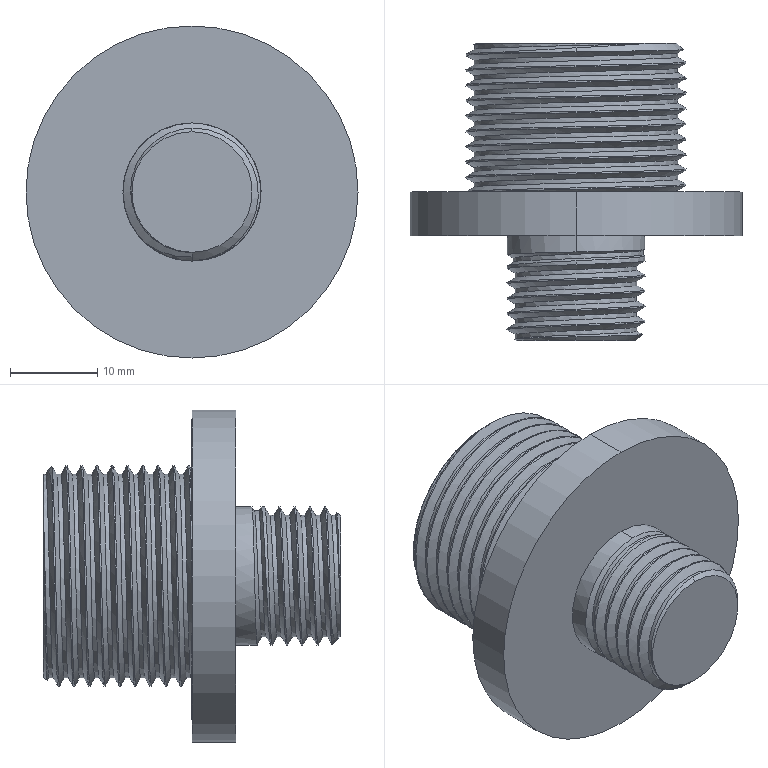Part | SolidWorks | features Helix 2, SweepCut 2, Revolution 1 | 1 solid | 51 faces | box 38 x 34 x 38 mm | volume 15399 mm3 | cylinder 32 | spline 7 | cone 6 | plane 6 | commonest cylinder face diameters 25.2 x19 15.8 x11 38 x2